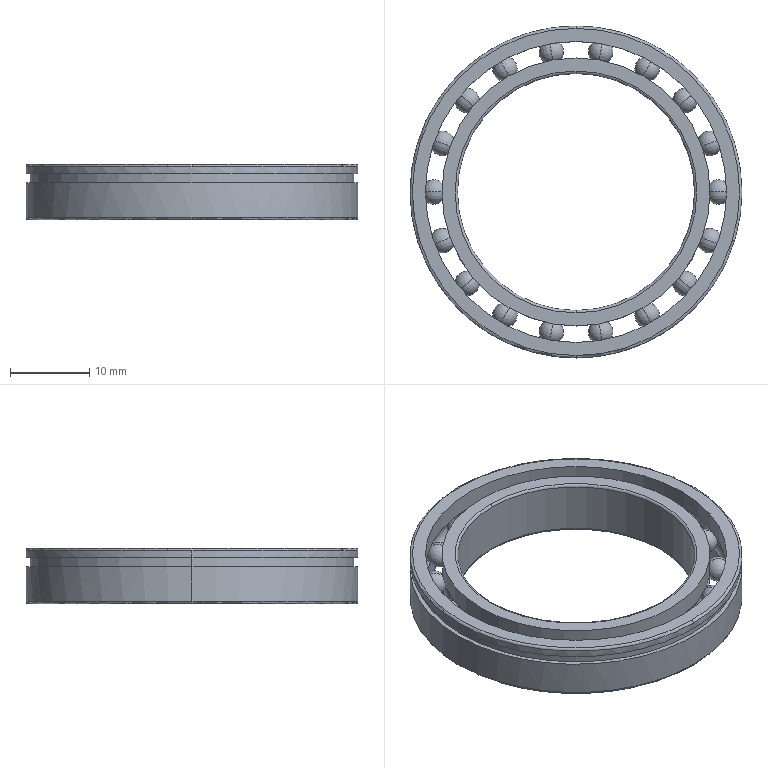Part | SolidWorks | 20 solids | 72 faces | box 42 x 42 x 7 mm | volume 3105 mm3 | sphere 36 | cylinder 16 | torus 14 | plane 6 | commonest cylinder face diameters 33.912 x4 38.088 x4 42 x4 30 x2 40.92 x2